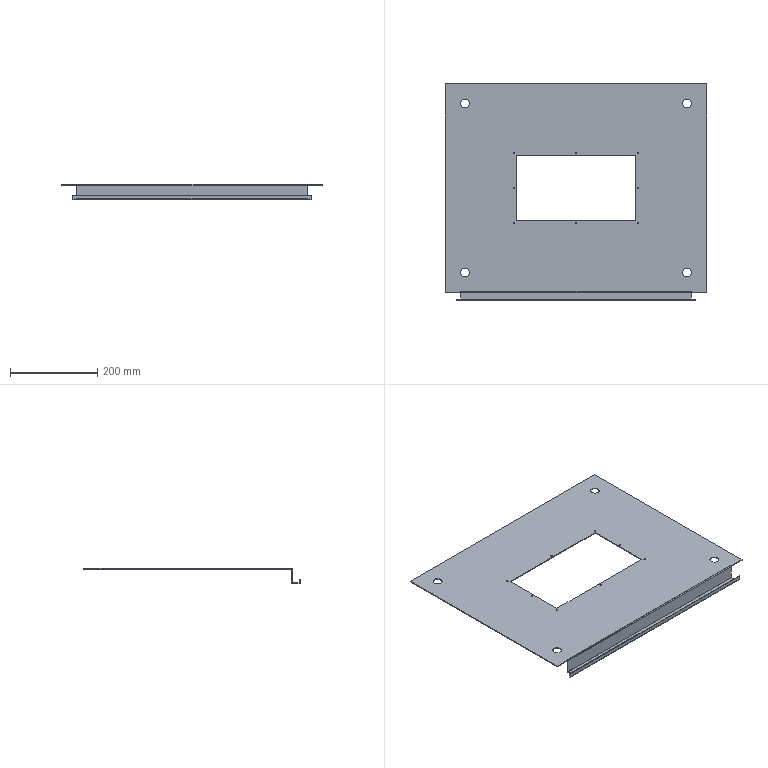Part | SolidWorks | features ICE 2, MoveFace 2, BaseBody 1 | 1 solid | 62 faces | box 600 x 496 x 35 mm | volume 549272 mm3 | plane 32 | cylinder 30 | commonest cylinder face diameters 4 x16 20 x8 0.2 x3 4.2 x3